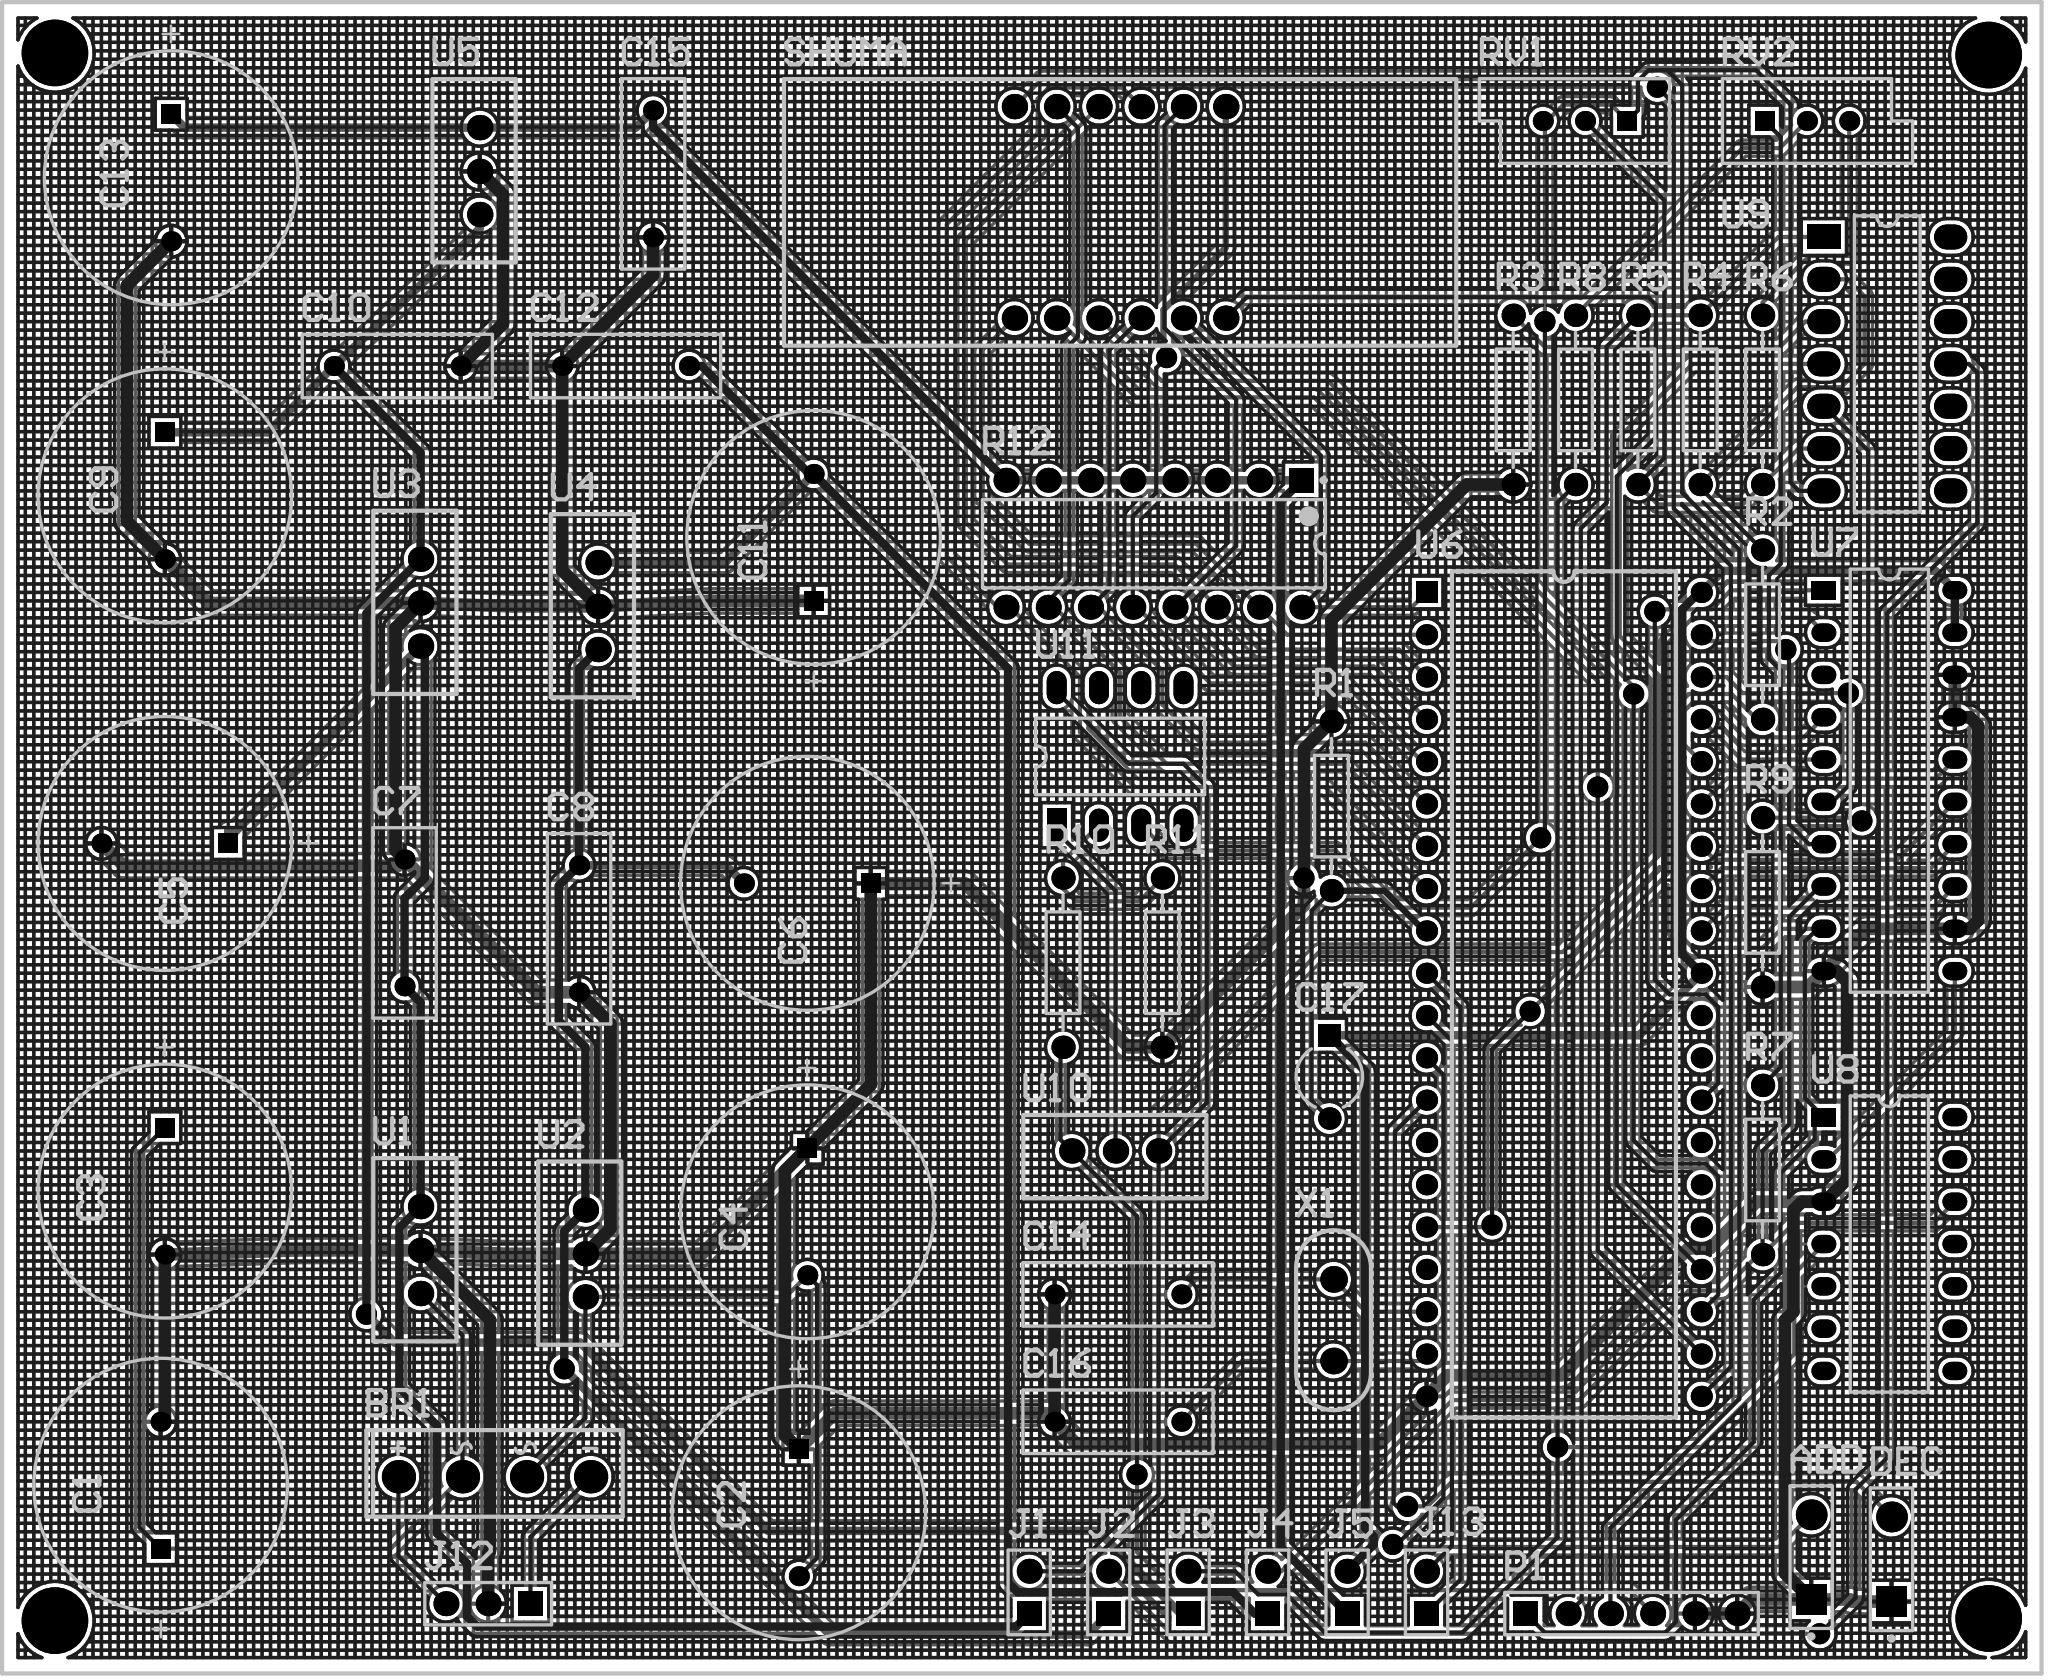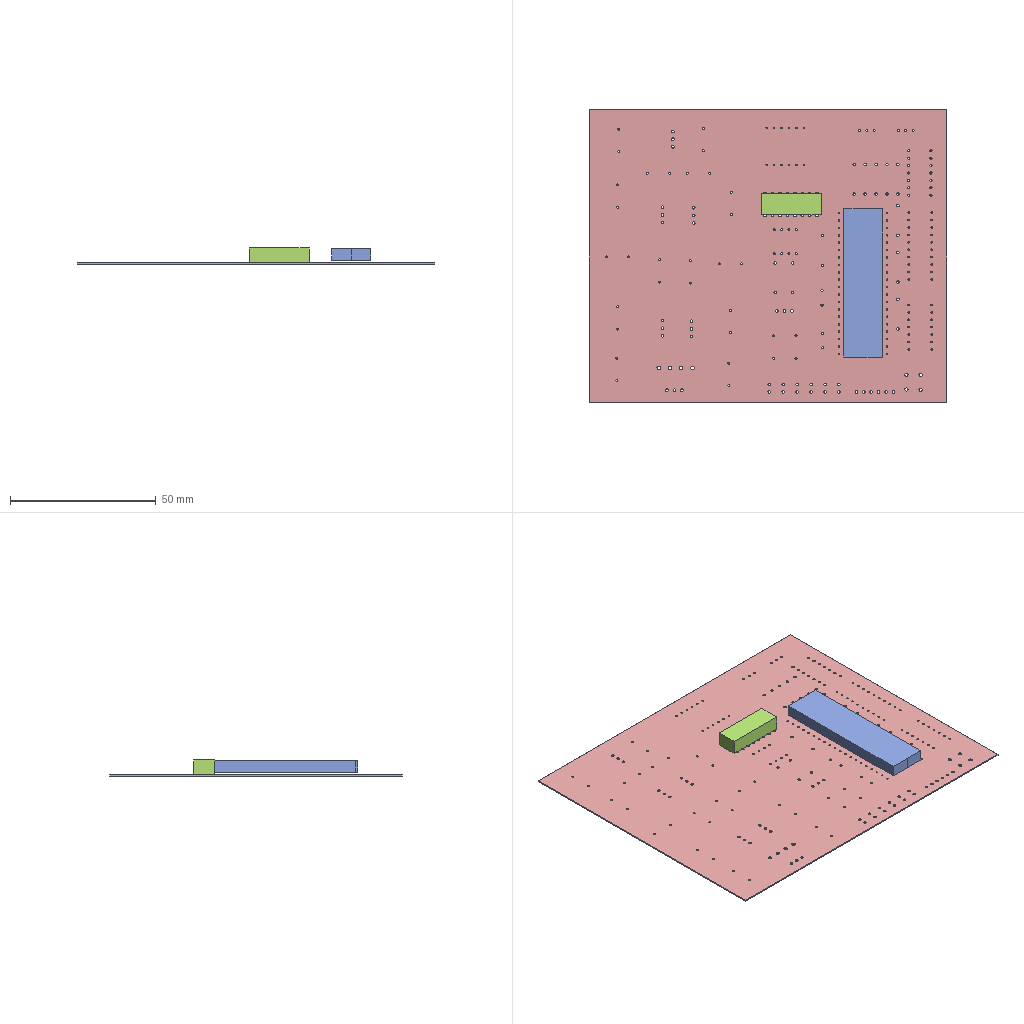Circuit board layout | Altium Designer | box 122.6 x 100.3 x 5.5 mm
Layer stack:
# Altium Designer layer stack of  (unit mm; dielectric type: 0 none, 1 core, 2 prepreg, 3 surface material)
index,name,kind,layer,copper_thickness_mm,dielectric_type,dielectric_thickness_mm,dielectric_material,dielectric_constant
0,Top Paste,other,,,,,,
1,Top Overlay,other,,,,,,
2,Top Solder,dielectric,,,3,0.0102,Solder Resist,3.5
3,Top Layer,copper,Top Layer,0.0356,,,,
4,Dielectric 1,dielectric,,,0,0.32,FR-4,4.8
5,Bottom Layer,copper,Bottom Layer,0.0356,,,,
6,Bottom Solder,dielectric,,,3,0.0102,Solder Resist,3.5
7,Bottom Overlay,other,,,,,,
8,Bottom Paste,other,,,,,,
# drill layer pairs: low layer,high layer
drill_pair,Top Layer,Bottom Layer
Part placement:
Designator,Comment,Layer,Footprint,Center-X(mm),Center-Y(mm),Rotation
C15,Cap,TopLayer,RAD-0.3,65.151,116.056,90
X1,Component_1,TopLayer,LC-HC-49S,106.045,47.244,90
U11,,TopLayer,NE5532,93.218,81.087,90
U10,7805,TopLayer,7805,92.922,57.404,180
U9,Component_1,TopLayer,TL084,139.319,104.648,0
U8,Component_1,TopLayer,LM324,139.444,51.816,360
U7,Component_1,TopLayer,DAC0832,139.444,79.629,360
U6,89c51,TopLayer,89c51,119.888,66.802,0
U5,7805,TopLayer,7805,54.737,116.225,90
U4,7809,TopLayer,7805,61.849,90.112,90
U3,7809,TopLayer,7805,51.181,90.317,90
U2,7818,TopLayer,7805,61.087,51.251,90
U1,7818,TopLayer,7805,51.181,51.455,90
SHUMA,Dpy Red-CA,TopLayer,四位数码管,93.218,113.744,180
RV2,RPot,TopLayer,VR5,134.493,119.231,360
RV1,RPot,TopLayer,VR5,121.158,119.231,180
R12,Res Pack2,TopLayer,DIP-16,95.25,93.853,270
R11,Res2,TopLayer,AXIAL-0.4,95.758,68.707,270
R10,Res2,TopLayer,AXIAL-0.4,89.789,68.707,90
R9,Res2,TopLayer,AXIAL-0.4,131.826,72.326,270
R8,Res2,TopLayer,AXIAL-0.4,120.587,102.489,90
R7,Res2,TopLayer,AXIAL-0.4,131.826,56.261,270
R6,Res2,TopLayer,AXIAL-0.4,131.826,102.489,90
R5,Res2,TopLayer,AXIAL-0.4,124.333,102.489,90
R4,Res2,TopLayer,AXIAL-0.4,128.079,102.489,90
R3,Res2,TopLayer,AXIAL-0.4,116.84,102.489,270
R2,Res2,TopLayer,AXIAL-0.4,131.826,88.392,270
R1,Res2,TopLayer,AXIAL-0.4,105.918,78.105,270
P1,Header 6,TopLayer,HDR1X6,123.952,29.633,360
J13,Header 2,TopLayer,HDR1X2,111.633,30.903,90
J12,Header 3,TopLayer,HDR1X3,55.245,30.226,180
J5,Header 2,TopLayer,HDR1X2,106.858,30.903,90
J4,Header 2,TopLayer,HDR1X2,102.083,30.903,90
J3,Header 2,TopLayer,HDR1X2,97.307,30.903,90
J2,Header 2,TopLayer,HDR1X2,92.532,30.903,90
J1,Header 2,TopLayer,HDR1X2,87.757,30.903,90
DEC,SW-PB,TopLayer,SPST-2,139.573,32.893,90
C17,Cap2,TopLayer,CAPR5-4X5,105.791,61.849,270
C16,Cap,TopLayer,RAD-0.3,93.091,41.148,360
C14,Cap,TopLayer,RAD-0.3,93.091,48.794,360
C13,Cap Pol1,TopLayer,RB7.6-15,36.195,115.824,90
C12,Cap,TopLayer,RAD-0.3,63.5,104.521,180
C11,Cap Pol1,TopLayer,RB7.6-15,74.803,94.234,270
C10,Cap,TopLayer,RAD-0.3,49.784,104.521,180
C9,Cap Pol1,TopLayer,RB7.6-15,35.814,96.733,90
C8,Cap,TopLayer,RAD-0.3,60.706,70.739,270
C7,Cap,TopLayer,RAD-0.3,50.218,71.093,270
C6,Cap Pol1,TopLayer,RB7.6-15,74.422,73.466,360
C5,Cap Pol1,TopLayer,RB7.6-15,35.814,75.864,360
C4,Cap Pol1,TopLayer,RB7.6-15,74.422,53.751,90
C3,Cap Pol1,TopLayer,RB7.6-15,35.814,54.995,90
C2,Cap Pol1,TopLayer,RB7.6-15,73.914,35.687,90
C1,Cap Pol1,TopLayer,RB7.6-15,35.56,37.338,270
BR1,Bridge1,TopLayer,LC-KBP,55.626,37.846,360
ADD,SW-PB,TopLayer,SPST-2,134.747,33.02,90
Pad and via stacks:
# Altium Designer via and pad stacks of  (unit mm). Each distinct definition once, with the count of objects using it.
# via: kind,start_layer,end_layer,hole_mm,diameter_mm,mode(0 simple;1 top-mid-bottom;2 full stack),diameter_per_layer,count,example_net
# pad: kind,layer,hole_mm,hole_type(0 round;1 square;2 slot),plating,top_size,top_shape(1 round;2 rect;3 octagon;9 rounded rect),mid_size,bottom_size,mode,footprint,size_per_layer,count,example
pad,Multi-Layer,0.7,0,plated,1.2x1.2,1,1.2x1.2,1.2x1.2,0,RAD-0.3,,14,C15.2
pad,Multi-Layer,0.9,0,plated,1.5x1.5,2,1.5x1.5,1.5x1.5,0,HDR1X2,,6,J13.1
pad,Multi-Layer,0.9,0,plated,1.5x1.5,1,1.5x1.5,1.5x1.5,0,HDR1X2,,6,J13.2
pad,Multi-Layer,0.75,0,plated,2x1.5,2,2x1.5,2x1.5,0,TL084,,1,U9.1
pad,Multi-Layer,0.75,0,plated,2x1.5,1,2x1.5,2x1.5,0,TL084,,13,U9.2
pad,Multi-Layer,1.1,0,plated,1.85x1.85,2,1.85x1.85,1.85x1.85,0,SPST-2,,2,ADD.1
pad,Multi-Layer,1.1,0,plated,1.85x1.85,1,1.85x1.85,1.85x1.85,0,SPST-2,,2,ADD.2
pad,Multi-Layer,0.7,0,plated,1.2x1.2,2,1.2x1.2,1.2x1.2,0,RB7.6-15,,9,C11.1
pad,Multi-Layer,0.7,0,plated,1.2x1.2,1,1.2x1.2,1.2x1.2,0,RB7.6-15,,9,C11.2
pad,Multi-Layer,0.91,0,plated,1.524x1.524,1,1.524x1.524,1.524x1.524,0,7805,,18,U5.1
pad,Multi-Layer,0.65,0,plated,2x1.2,1,2x1.2,2x1.2,0,NE5532,,7,U11.5
pad,Multi-Layer,0.65,0,plated,2x1.2,2,2x1.2,2x1.2,0,NE5532,,1,U11.1
pad,Multi-Layer,1.2,0,plated,2x2,1,2x2,2x2,0,LC-KBP,,4,BR1.3
pad,Multi-Layer,0.85,0,plated,1.4x1.4,1,1.4x1.4,1.4x1.4,0,AXIAL-0.4,,22,R10.1
pad,Multi-Layer,0.9,0,plated,1.5x1.5,2,1.5x1.5,1.5x1.5,0,HDR1X3,,1,J12.1
pad,Multi-Layer,0.9,0,plated,1.5x1.5,1,1.5x1.5,1.5x1.5,0,HDR1X3,,2,J12.2
pad,Multi-Layer,0.55,0,plated,1.5x1.1,2,1.5x1.1,1.5x1.1,0,DAC0832,,1,U7.1
pad,Multi-Layer,0.55,0,plated,1.5x1.1,1,1.5x1.1,1.5x1.1,0,DAC0832,,19,U7.2
pad,Multi-Layer,0.51,0,plated,1.524x1.524,1,1.524x1.524,1.524x1.524,0,\u00CB\u00C4\u00CE\u00BB\u00CA\u00FD\u00C2\u00EB\u00B9\u00DC,,12,SHUMA.1
pad,Multi-Layer,0.5588,0,plated,1.27x1.27,2,1.27x1.27,1.27x1.27,0,89c51,,1,U6.1
pad,Multi-Layer,0.5588,0,plated,1.27x1.27,1,1.27x1.27,1.27x1.27,0,89c51,,39,U6.2
pad,Multi-Layer,0.9,0,plated,1.5x1.5,1,1.5x1.5,1.5x1.5,0,DIP-16,,15,R12.9
pad,Multi-Layer,0.9,0,plated,1.5x1.5,2,1.5x1.5,1.5x1.5,0,DIP-16,,1,R12.1
pad,Multi-Layer,0.55,0,plated,1.5x1.1,2,1.5x1.1,1.5x1.1,0,LM324,,1,U8.1
pad,Multi-Layer,0.55,0,plated,1.5x1.1,1,1.5x1.1,1.5x1.1,0,LM324,,13,U8.2
pad,Multi-Layer,0.8,0,plated,1.35x1.35,1,1.35x1.35,1.35x1.35,0,CAPR5-4X5,,1,C17.2
pad,Multi-Layer,0.8,0,plated,1.35x1.35,2,1.35x1.35,1.35x1.35,0,CAPR5-4X5,,1,C17.1
pad,Multi-Layer,0.7,0,plated,1.2x1.2,2,1.2x1.2,1.2x1.2,0,VR5,,2,RV2.1
pad,Multi-Layer,0.7,0,plated,1.2x1.2,1,1.2x1.2,1.2x1.2,0,VR5,,4,RV2.2
pad,Multi-Layer,0.9,0,plated,1.5x1.5,2,1.5x1.5,1.5x1.5,0,HDR1X6,,1,P1.1
pad,Multi-Layer,0.9,0,plated,1.5x1.5,1,1.5x1.5,1.5x1.5,0,HDR1X6,,5,P1.2
pad,Multi-Layer,0.7,0,plated,1.6x1.6,1,1.6x1.6,1.6x1.6,0,LC-HC-49S,,2,X1.1
via,Top Layer,Bottom Layer,0.7112,1.27,0,,20,P27
via,Top Layer,Bottom Layer,3,4,0,,4,
Copper pours:
name,layer,net,type(0 solid;1 hatched;2 none)
Top Layer-No Net,Top Layer,T2,0
Top Layer-No Net,Bottom Layer,T2,0
Design rules, without the lines most boards share:
# Altium Designer design rules of  (exported by Altium Designer, unit mm)
# columns: name | kind | enabled | priority | scope1 | scope2 | descriptor | typed fields (field=value)
VCC_5 | 2 | enabled | 7 | InNet('-18V') | All | Width Constraint (Min=10mil) (Max=25mil) (Preferred=20mil) (InNet('-18V')) |
VCC_4 | 2 | enabled | 6 | InNet('-9V') | All | Width Constraint (Min=10mil) (Max=25mil) (Preferred=20mil) (InNet('-9V')) |
VCC_3 | 2 | enabled | 5 | InNet('+18V') | All | Width Constraint (Min=10mil) (Max=25mil) (Preferred=20mil) (InNet('+18V')) |
VCC_2 | 2 | enabled | 4 | InNet('+9V') | All | Width Constraint (Min=10mil) (Max=25mil) (Preferred=20mil) (InNet('+9V')) |
VCC_1 | 2 | enabled | 3 | InNet('+5V') | All | Width Constraint (Min=10mil) (Max=25mil) (Preferred=20mil) (InNet('+5V')) |
GND | 2 | enabled | 1 | InNet('T2') | All | Width Constraint (Min=20mil) (Max=35mil) (Preferred=30mil) (InNet('T2')) |
VCC | 2 | enabled | 2 | InNet('VCC') | All | Width Constraint (Min=10mil) (Max=25mil) (Preferred=20mil) (InNet('VCC')) |
Clearance | 0 | enabled | 1 | All | All | Clearance Constraint (Gap=10mil) (All),(All) | gap=0.254
PlaneConnect | 6 | enabled | 1 | All | All | Power Plane Connect Rule(Relief Connect )(Expansion=20mil) (Conductor Width=10mil) (Air Gap=10mil) (Entries=4) (All) | relief_conductor_width=0.254 relief_entries=4 relief_expansion=0.508
PolygonConnect | 20 | enabled | 1 | All | All | Polygon Connect Rule(Relief Connect )(Conductor Width=10mil) (Relief Angle=90 Angle) (Entries=4) (Air Gap Width=10mil) (All),(All) | connect_style(0=relief,1=direct,2=none)=0 relief_conductor_width=0.254 relief_entries=4
Width | 2 | enabled | 8 | All | All | Width Constraint (Min=8mil) (Max=15mil) (Preferred=10mil) (All) |
RoutingVias | 11 | enabled | 1 | All | All | Routing Via (MinHoleWidth=28mil) (MaxHoleWidth=28mil) (PreferredHoleWidth=28mil) (MinWidth=50mil) (MaxWidth=50mil) (PreferedWidth=50mil) (All) | via_min_hole=0.7112 via_max_hole=0.7112 via_preferred_diameter=1.27 via_preferred_hole=0.7112
PasteMaskExpansion | 14 | enabled | 1 | All | All | Paste Mask Expansion (Expansion =0mil) (All) | expansion=0
SolderMaskExpansion | 13 | enabled | 1 | All | All | Solder Mask Expansion (Expansion =4mil) (All) | expansion=0.1016
HoleSize | 42 | enabled | 1 | All | All | Hole Size Constraint (Min=1mil) (Max=500mil) (All) |
DiffPairsRouting | 51 | enabled | 1 | All | All | Differential Pairs Uncoupled Length using the Gap Constraints (Min=10mil) (Max=10mil) (Prefered=10mil)  and Width Constraints (Min=15mil) (Max=15mil) (Prefered=15mil) (All) |
HoleToHoleClearance | 52 | enabled | 1 | All | All | Hole To Hole Clearance (Gap=10mil) (All),(All) | gap=0.254
SilkToSolderMaskClearance | 54 | enabled | 1 | IsPad | All | Silk To Solder Mask (Clearance=0mil) (IsPad),(All) |